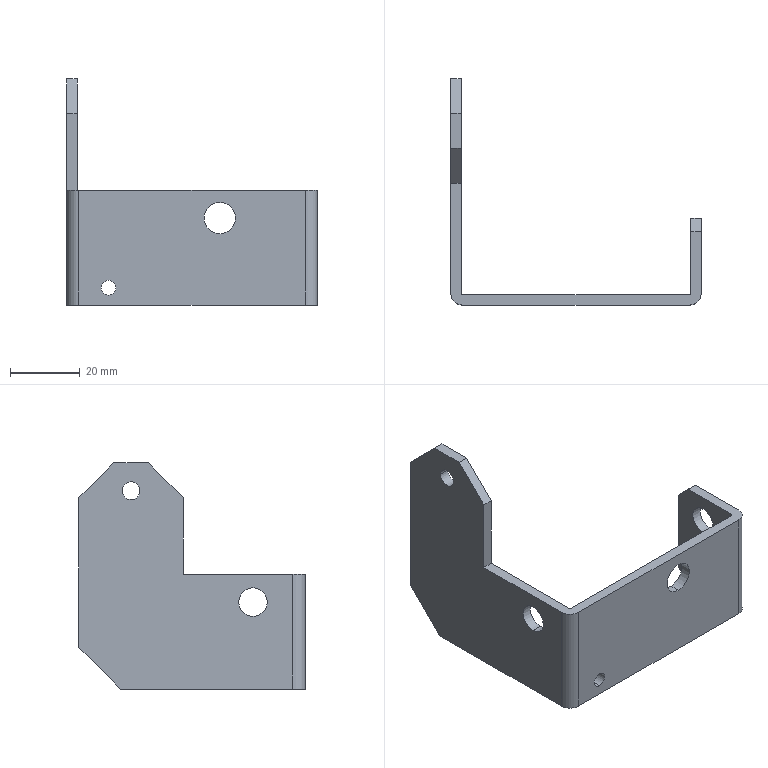Part | STEP file | 8XS161060 | 1 solid | 35 faces | box 72 x 65 x 65 mm | volume 16979 mm3 | plane 21 | cylinder 14 | commonest cylinder face diameters 8.2 x4 1 x2 4.242 x2 5.1 x2 7 x2 9 x2